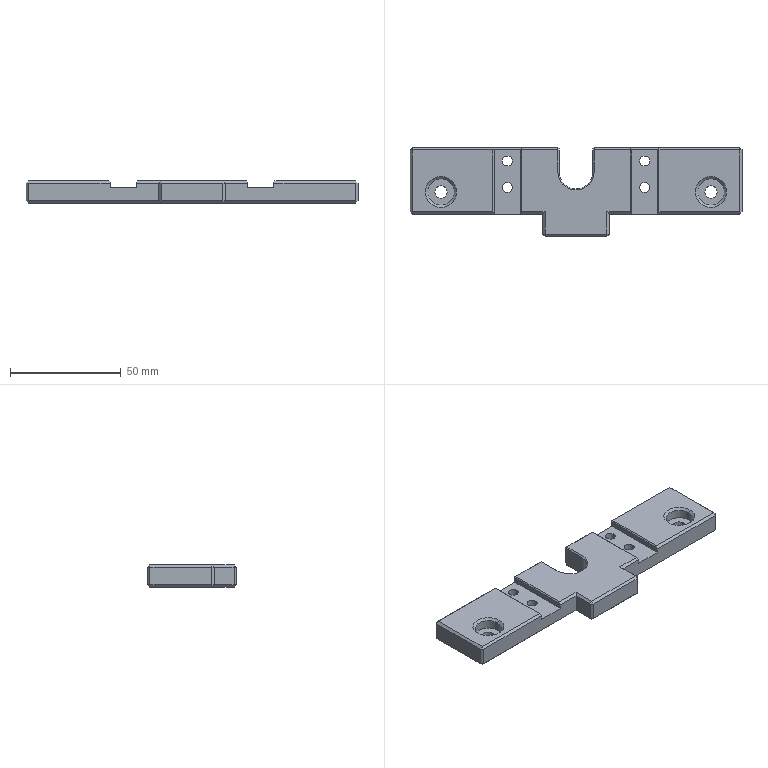Part | STEP file | BPSP-11-13 Rotary Support Plate_Default | 1 solid | 106 faces | box 150 x 40 x 10 mm | volume 40974 mm3 | plane 83 | cylinder 17 | cone 6 | commonest cylinder face diameters 4.5 x8 5.5 x4 12 x4 15.3 x1